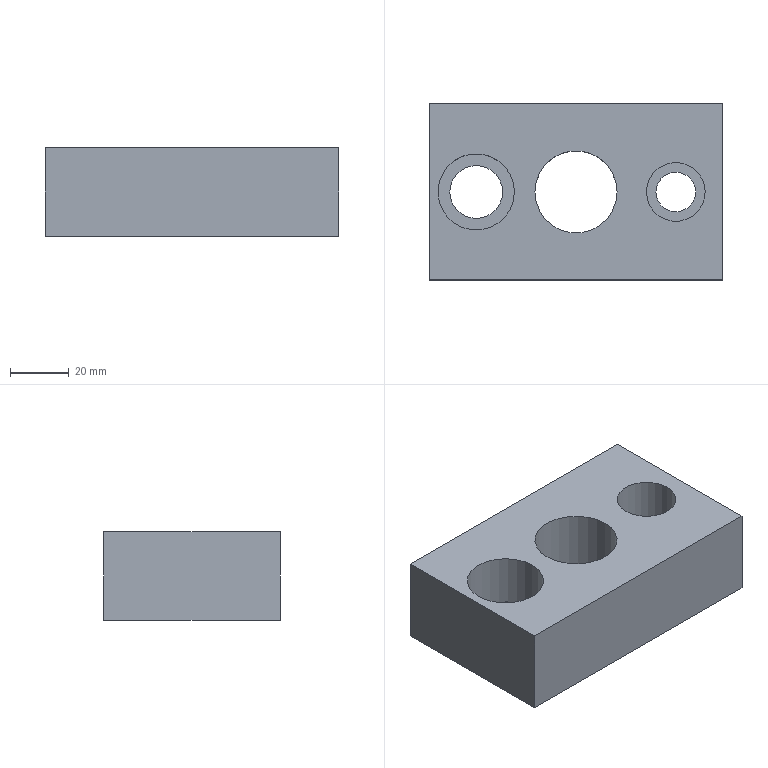Part | STEP file | lll_id4438_x_t | 1 solid | 15 faces | box 100 x 60 x 30 mm | volume 135633 mm3 | plane 9 | cylinder 6 | commonest cylinder face diameters 13.509 x1 18.009 x1 20.008 x1 26.008 x1 28 x1 40 x1
STEP:
#1=CARTESIAN_POINT('',(3051.995,87.,-68.));
#2=VERTEX_POINT('',#1);
#3=CARTESIAN_POINT('',(3061.,87.,-68.));
#4=DIRECTION('',(0.,0.,-1.));
#5=DIRECTION('',(-1.,0.,0.));
#6=AXIS2_PLACEMENT_3D('',#3,#4,#5);
#7=CIRCLE('',#6,9.005);
#8=EDGE_CURVE('',#2,#2,#7,.T.);
#9=ORIENTED_EDGE('',*,*,#8,.F.);
#10=EDGE_LOOP('',(#9));
#11=FACE_BOUND('',#10,.T.);
#12=CARTESIAN_POINT('',(3051.995,87.,-80.));
#13=VERTEX_POINT('',#12);
#14=CARTESIAN_POINT('',(3061.,87.,-80.));
#15=DIRECTION('',(0.,0.,-1.));
#16=DIRECTION('',(-1.,0.,0.));
#17=AXIS2_PLACEMENT_3D('',#14,#15,#16);
#18=CIRCLE('',#17,9.005);
#19=EDGE_CURVE('',#13,#13,#18,.T.);
#20=ORIENTED_EDGE('',*,*,#19,.T.);
#21=EDGE_LOOP('',(#20));
#22=FACE_BOUND('',#21,.T.);
#23=CARTESIAN_POINT('',(3061.,87.,-49.));
#24=DIRECTION('',(0.,0.,-1.));
#25=DIRECTION('',(-1.,0.,0.));
#26=AXIS2_PLACEMENT_3D('',#23,#24,#25);
#27=CYLINDRICAL_SURFACE('',#26,9.005);
#28=ADVANCED_FACE('',(#11,#22),#27,.F.);
#29=CARTESIAN_POINT('',(3074.004,87.,-50.));
#30=VERTEX_POINT('',#29);
#31=CARTESIAN_POINT('',(3061.,87.,-50.));
#32=DIRECTION('',(0.,0.,1.));
#33=DIRECTION('',(1.,0.,0.));
#34=AXIS2_PLACEMENT_3D('',#31,#32,#33);
#35=CIRCLE('',#34,13.004);
#36=EDGE_CURVE('',#30,#30,#35,.T.);
#37=ORIENTED_EDGE('',*,*,#36,.F.);
#38=EDGE_LOOP('',(#37));
#39=FACE_BOUND('',#38,.T.);
#40=CARTESIAN_POINT('',(3081.,87.,-50.));
#41=VERTEX_POINT('',#40);
#42=CARTESIAN_POINT('',(3095.,87.,-50.));
#43=DIRECTION('',(0.,0.,-1.));
#44=DIRECTION('',(-1.,0.,0.));
#45=AXIS2_PLACEMENT_3D('',#42,#43,#44);
#46=CIRCLE('',#45,14.);
#47=EDGE_CURVE('',#41,#41,#46,.T.);
#48=ORIENTED_EDGE('',*,*,#47,.T.);
#49=EDGE_LOOP('',(#48));
#50=FACE_BOUND('',#49,.T.);
#51=CARTESIAN_POINT('',(3118.996,87.,-50.));
#52=VERTEX_POINT('',#51);
#53=CARTESIAN_POINT('',(3129.,87.,-50.));
#54=DIRECTION('',(0.,0.,1.));
#55=DIRECTION('',(-1.,0.,0.));
#56=AXIS2_PLACEMENT_3D('',#53,#54,#55);
#57=CIRCLE('',#56,10.004);
#58=EDGE_CURVE('',#52,#52,#57,.T.);
#59=ORIENTED_EDGE('',*,*,#58,.F.);
#60=EDGE_LOOP('',(#59));
#61=FACE_BOUND('',#60,.T.);
#62=CARTESIAN_POINT('',(3045.,57.,-50.));
#63=VERTEX_POINT('',#62);
#64=CARTESIAN_POINT('',(3145.,57.,-50.));
#65=VERTEX_POINT('',#64);
#66=CARTESIAN_POINT('',(3095.,57.,-50.));
#67=DIRECTION('',(1.,0.,0.));
#68=VECTOR('',#67,1.);
#69=LINE('',#66,#68);
#70=EDGE_CURVE('',#63,#65,#69,.T.);
#71=ORIENTED_EDGE('',*,*,#70,.T.);
#72=CARTESIAN_POINT('',(3145.,117.,-50.));
#73=VERTEX_POINT('',#72);
#74=CARTESIAN_POINT('',(3145.,87.,-50.));
#75=DIRECTION('',(0.,1.,0.));
#76=VECTOR('',#75,1.);
#77=LINE('',#74,#76);
#78=EDGE_CURVE('',#65,#73,#77,.T.);
#79=ORIENTED_EDGE('',*,*,#78,.T.);
#80=CARTESIAN_POINT('',(3045.,117.,-50.));
#81=VERTEX_POINT('',#80);
#82=CARTESIAN_POINT('',(3095.,117.,-50.));
#83=DIRECTION('',(-1.,0.,0.));
#84=VECTOR('',#83,1.);
#85=LINE('',#82,#84);
#86=EDGE_CURVE('',#73,#81,#85,.T.);
#87=ORIENTED_EDGE('',*,*,#86,.T.);
#88=CARTESIAN_POINT('',(3045.,87.,-50.));
#89=DIRECTION('',(0.,-1.,0.));
#90=VECTOR('',#89,1.);
#91=LINE('',#88,#90);
#92=EDGE_CURVE('',#81,#63,#91,.T.);
#93=ORIENTED_EDGE('',*,*,#92,.T.);
#94=EDGE_LOOP('',(#71,#79,#87,#93));
#95=FACE_BOUND('',#94,.T.);
#96=CARTESIAN_POINT('',(3095.,87.,-50.));
#97=DIRECTION('',(0.,0.,1.));
#98=DIRECTION('',(-1.,0.,0.));
#99=AXIS2_PLACEMENT_3D('',#96,#97,#98);
#100=PLANE('',#99);
#101=ADVANCED_FACE('',(#39,#50,#61,#95),#100,.T.);
#102=CARTESIAN_POINT('',(3045.,57.,-80.));
#103=VERTEX_POINT('',#102);
#104=CARTESIAN_POINT('',(3045.,57.,-80.));
#105=DIRECTION('',(0.,0.,1.));
#106=VECTOR('',#105,1.);
#107=LINE('',#104,#106);
#108=EDGE_CURVE('',#103,#63,#107,.T.);
#109=ORIENTED_EDGE('',*,*,#108,.F.);
#110=CARTESIAN_POINT('',(3145.,57.,-80.));
#111=VERTEX_POINT('',#110);
#112=CARTESIAN_POINT('',(3095.,57.,-80.));
#113=DIRECTION('',(-1.,0.,0.));
#114=VECTOR('',#113,1.);
#115=LINE('',#112,#114);
#116=EDGE_CURVE('',#111,#103,#115,.T.);
#117=ORIENTED_EDGE('',*,*,#116,.F.);
#118=CARTESIAN_POINT('',(3145.,57.,-80.));
#119=DIRECTION('',(0.,0.,1.));
#120=VECTOR('',#119,1.);
#121=LINE('',#118,#120);
#122=EDGE_CURVE('',#111,#65,#121,.T.);
#123=ORIENTED_EDGE('',*,*,#122,.T.);
#124=ORIENTED_EDGE('',*,*,#70,.F.);
#125=EDGE_LOOP('',(#109,#117,#123,#124));
#126=FACE_OUTER_BOUND('',#125,.T.);
#127=CARTESIAN_POINT('',(3095.,57.,-80.));
#128=DIRECTION('',(0.,-1.,0.));
#129=DIRECTION('',(0.,0.,-1.));
#130=AXIS2_PLACEMENT_3D('',#127,#128,#129);
#131=PLANE('',#130);
#132=ADVANCED_FACE('',(#126),#131,.T.);
#133=ORIENTED_EDGE('',*,*,#122,.F.);
#134=CARTESIAN_POINT('',(3145.,117.,-80.));
#135=VERTEX_POINT('',#134);
#136=CARTESIAN_POINT('',(3145.,87.,-80.));
#137=DIRECTION('',(0.,-1.,0.));
#138=VECTOR('',#137,1.);
#139=LINE('',#136,#138);
#140=EDGE_CURVE('',#135,#111,#139,.T.);
#141=ORIENTED_EDGE('',*,*,#140,.F.);
#142=CARTESIAN_POINT('',(3145.,117.,-80.));
#143=DIRECTION('',(0.,0.,1.));
#144=VECTOR('',#143,1.);
#145=LINE('',#142,#144);
#146=EDGE_CURVE('',#135,#73,#145,.T.);
#147=ORIENTED_EDGE('',*,*,#146,.T.);
#148=ORIENTED_EDGE('',*,*,#78,.F.);
#149=EDGE_LOOP('',(#133,#141,#147,#148));
#150=FACE_OUTER_BOUND('',#149,.T.);
#151=CARTESIAN_POINT('',(3145.,87.,-80.));
#152=DIRECTION('',(1.,0.,0.));
#153=DIRECTION('',(0.,0.,1.));
#154=AXIS2_PLACEMENT_3D('',#151,#152,#153);
#155=PLANE('',#154);
#156=ADVANCED_FACE('',(#150),#155,.T.);
#157=ORIENTED_EDGE('',*,*,#146,.F.);
#158=CARTESIAN_POINT('',(3045.,117.,-80.));
#159=VERTEX_POINT('',#158);
#160=CARTESIAN_POINT('',(3095.,117.,-80.));
#161=DIRECTION('',(1.,0.,0.));
#162=VECTOR('',#161,1.);
#163=LINE('',#160,#162);
#164=EDGE_CURVE('',#159,#135,#163,.T.);
#165=ORIENTED_EDGE('',*,*,#164,.F.);
#166=CARTESIAN_POINT('',(3045.,117.,-80.));
#167=DIRECTION('',(0.,0.,1.));
#168=VECTOR('',#167,1.);
#169=LINE('',#166,#168);
#170=EDGE_CURVE('',#159,#81,#169,.T.);
#171=ORIENTED_EDGE('',*,*,#170,.T.);
#172=ORIENTED_EDGE('',*,*,#86,.F.);
#173=EDGE_LOOP('',(#157,#165,#171,#172));
#174=FACE_OUTER_BOUND('',#173,.T.);
#175=CARTESIAN_POINT('',(3095.,117.,-80.));
#176=DIRECTION('',(0.,1.,0.));
#177=DIRECTION('',(0.,0.,1.));
#178=AXIS2_PLACEMENT_3D('',#175,#176,#177);
#179=PLANE('',#178);
#180=ADVANCED_FACE('',(#174),#179,.T.);
#181=ORIENTED_EDGE('',*,*,#19,.F.);
#182=EDGE_LOOP('',(#181));
#183=FACE_BOUND('',#182,.T.);
#184=CARTESIAN_POINT('',(3135.755,87.,-80.));
#185=VERTEX_POINT('',#184);
#186=CARTESIAN_POINT('',(3129.,87.,-80.));
#187=DIRECTION('',(0.,0.,1.));
#188=DIRECTION('',(1.,0.,0.));
#189=AXIS2_PLACEMENT_3D('',#186,#187,#188);
#190=CIRCLE('',#189,6.755);
#191=EDGE_CURVE('',#185,#185,#190,.T.);
#192=ORIENTED_EDGE('',*,*,#191,.T.);
#193=EDGE_LOOP('',(#192));
#194=FACE_BOUND('',#193,.T.);
#195=CARTESIAN_POINT('',(3115.,87.,-80.));
#196=VERTEX_POINT('',#195);
#197=CARTESIAN_POINT('',(3095.,87.,-80.));
#198=DIRECTION('',(0.,0.,1.));
#199=DIRECTION('',(1.,0.,0.));
#200=AXIS2_PLACEMENT_3D('',#197,#198,#199);
#201=CIRCLE('',#200,20.);
#202=EDGE_CURVE('',#196,#196,#201,.T.);
#203=ORIENTED_EDGE('',*,*,#202,.T.);
#204=EDGE_LOOP('',(#203));
#205=FACE_BOUND('',#204,.T.);
#206=CARTESIAN_POINT('',(3045.,87.,-80.));
#207=DIRECTION('',(0.,1.,0.));
#208=VECTOR('',#207,1.);
#209=LINE('',#206,#208);
#210=EDGE_CURVE('',#103,#159,#209,.T.);
#211=ORIENTED_EDGE('',*,*,#210,.T.);
#212=ORIENTED_EDGE('',*,*,#164,.T.);
#213=ORIENTED_EDGE('',*,*,#140,.T.);
#214=ORIENTED_EDGE('',*,*,#116,.T.);
#215=EDGE_LOOP('',(#211,#212,#213,#214));
#216=FACE_BOUND('',#215,.T.);
#217=CARTESIAN_POINT('',(3095.,87.,-80.));
#218=DIRECTION('',(0.,0.,-1.));
#219=DIRECTION('',(1.,0.,0.));
#220=AXIS2_PLACEMENT_3D('',#217,#218,#219);
#221=PLANE('',#220);
#222=ADVANCED_FACE('',(#183,#194,#205,#216),#221,.T.);
#223=ORIENTED_EDGE('',*,*,#210,.F.);
#224=ORIENTED_EDGE('',*,*,#108,.T.);
#225=ORIENTED_EDGE('',*,*,#92,.F.);
#226=ORIENTED_EDGE('',*,*,#170,.F.);
#227=EDGE_LOOP('',(#223,#224,#225,#226));
#228=FACE_OUTER_BOUND('',#227,.T.);
#229=CARTESIAN_POINT('',(3045.,87.,-80.));
#230=DIRECTION('',(-1.,0.,0.));
#231=DIRECTION('',(0.,0.,-1.));
#232=AXIS2_PLACEMENT_3D('',#229,#230,#231);
#233=PLANE('',#232);
#234=ADVANCED_FACE('',(#228),#233,.T.);
#235=CARTESIAN_POINT('',(3081.,87.,-70.));
#236=VERTEX_POINT('',#235);
#237=CARTESIAN_POINT('',(3095.,87.,-70.));
#238=DIRECTION('',(0.,0.,-1.));
#239=DIRECTION('',(1.,0.,0.));
#240=AXIS2_PLACEMENT_3D('',#237,#238,#239);
#241=CIRCLE('',#240,14.);
#242=EDGE_CURVE('',#236,#236,#241,.T.);
#243=ORIENTED_EDGE('',*,*,#242,.F.);
#244=EDGE_LOOP('',(#243));
#245=FACE_BOUND('',#244,.T.);
#246=CARTESIAN_POINT('',(3075.,87.,-70.));
#247=VERTEX_POINT('',#246);
#248=CARTESIAN_POINT('',(3095.,87.,-70.));
#249=DIRECTION('',(0.,0.,-1.));
#250=DIRECTION('',(1.,0.,0.));
#251=AXIS2_PLACEMENT_3D('',#248,#249,#250);
#252=CIRCLE('',#251,20.);
#253=EDGE_CURVE('',#247,#247,#252,.T.);
#254=ORIENTED_EDGE('',*,*,#253,.T.);
#255=EDGE_LOOP('',(#254));
#256=FACE_BOUND('',#255,.T.);
#257=CARTESIAN_POINT('',(3095.,87.,-70.));
#258=DIRECTION('',(0.,0.,1.));
#259=DIRECTION('',(-1.,0.,0.));
#260=AXIS2_PLACEMENT_3D('',#257,#258,#259);
#261=PLANE('',#260);
#262=ADVANCED_FACE('',(#245,#256),#261,.F.);
#263=ORIENTED_EDGE('',*,*,#202,.F.);
#264=EDGE_LOOP('',(#263));
#265=FACE_BOUND('',#264,.T.);
#266=ORIENTED_EDGE('',*,*,#253,.F.);
#267=EDGE_LOOP('',(#266));
#268=FACE_BOUND('',#267,.T.);
#269=CARTESIAN_POINT('',(3095.,87.,-75.));
#270=DIRECTION('',(0.,0.,-1.));
#271=DIRECTION('',(-1.,0.,0.));
#272=AXIS2_PLACEMENT_3D('',#269,#270,#271);
#273=CYLINDRICAL_SURFACE('',#272,20.);
#274=ADVANCED_FACE('',(#265,#268),#273,.F.);
#275=ORIENTED_EDGE('',*,*,#191,.F.);
#276=EDGE_LOOP('',(#275));
#277=FACE_BOUND('',#276,.T.);
#278=CARTESIAN_POINT('',(3135.755,87.,-65.));
#279=VERTEX_POINT('',#278);
#280=CARTESIAN_POINT('',(3129.,87.,-65.));
#281=DIRECTION('',(0.,0.,1.));
#282=DIRECTION('',(1.,0.,0.));
#283=AXIS2_PLACEMENT_3D('',#280,#281,#282);
#284=CIRCLE('',#283,6.755);
#285=EDGE_CURVE('',#279,#279,#284,.T.);
#286=ORIENTED_EDGE('',*,*,#285,.T.);
#287=EDGE_LOOP('',(#286));
#288=FACE_BOUND('',#287,.T.);
#289=CARTESIAN_POINT('',(3129.,87.,-48.));
#290=DIRECTION('',(0.,0.,-1.));
#291=DIRECTION('',(-1.,0.,0.));
#292=AXIS2_PLACEMENT_3D('',#289,#290,#291);
#293=CYLINDRICAL_SURFACE('',#292,6.755);
#294=ADVANCED_FACE('',(#277,#288),#293,.F.);
#295=ORIENTED_EDGE('',*,*,#285,.F.);
#296=EDGE_LOOP('',(#295));
#297=FACE_BOUND('',#296,.T.);
#298=CARTESIAN_POINT('',(3118.996,87.,-65.));
#299=VERTEX_POINT('',#298);
#300=CARTESIAN_POINT('',(3129.,87.,-65.));
#301=DIRECTION('',(0.,0.,1.));
#302=DIRECTION('',(-1.,0.,0.));
#303=AXIS2_PLACEMENT_3D('',#300,#301,#302);
#304=CIRCLE('',#303,10.004);
#305=EDGE_CURVE('',#299,#299,#304,.T.);
#306=ORIENTED_EDGE('',*,*,#305,.T.);
#307=EDGE_LOOP('',(#306));
#308=FACE_BOUND('',#307,.T.);
#309=CARTESIAN_POINT('',(3129.,87.,-65.));
#310=DIRECTION('',(0.,0.,-1.));
#311=DIRECTION('',(1.,0.,0.));
#312=AXIS2_PLACEMENT_3D('',#309,#310,#311);
#313=PLANE('',#312);
#314=ADVANCED_FACE('',(#297,#308),#313,.F.);
#315=ORIENTED_EDGE('',*,*,#305,.F.);
#316=EDGE_LOOP('',(#315));
#317=FACE_BOUND('',#316,.T.);
#318=ORIENTED_EDGE('',*,*,#58,.T.);
#319=EDGE_LOOP('',(#318));
#320=FACE_BOUND('',#319,.T.);
#321=CARTESIAN_POINT('',(3129.,87.,-50.));
#322=DIRECTION('',(0.,0.,-1.));
#323=DIRECTION('',(-1.,0.,0.));
#324=AXIS2_PLACEMENT_3D('',#321,#322,#323);
#325=CYLINDRICAL_SURFACE('',#324,10.004);
#326=ADVANCED_FACE('',(#317,#320),#325,.F.);
#327=ORIENTED_EDGE('',*,*,#47,.F.);
#328=EDGE_LOOP('',(#327));
#329=FACE_BOUND('',#328,.T.);
#330=ORIENTED_EDGE('',*,*,#242,.T.);
#331=EDGE_LOOP('',(#330));
#332=FACE_BOUND('',#331,.T.);
#333=CARTESIAN_POINT('',(3095.,87.,-8.));
#334=DIRECTION('',(0.,0.,-1.));
#335=DIRECTION('',(-1.,0.,0.));
#336=AXIS2_PLACEMENT_3D('',#333,#334,#335);
#337=CYLINDRICAL_SURFACE('',#336,14.);
#338=ADVANCED_FACE('',(#329,#332),#337,.F.);
#339=ORIENTED_EDGE('',*,*,#8,.T.);
#340=EDGE_LOOP('',(#339));
#341=FACE_BOUND('',#340,.T.);
#342=CARTESIAN_POINT('',(3074.004,87.,-68.));
#343=VERTEX_POINT('',#342);
#344=CARTESIAN_POINT('',(3061.,87.,-68.));
#345=DIRECTION('',(0.,0.,-1.));
#346=DIRECTION('',(1.,0.,0.));
#347=AXIS2_PLACEMENT_3D('',#344,#345,#346);
#348=CIRCLE('',#347,13.004);
#349=EDGE_CURVE('',#343,#343,#348,.T.);
#350=ORIENTED_EDGE('',*,*,#349,.F.);
#351=EDGE_LOOP('',(#350));
#352=FACE_BOUND('',#351,.T.);
#353=CARTESIAN_POINT('',(3061.,87.,-68.));
#354=DIRECTION('',(0.,0.,-1.));
#355=DIRECTION('',(1.,0.,0.));
#356=AXIS2_PLACEMENT_3D('',#353,#354,#355);
#357=PLANE('',#356);
#358=ADVANCED_FACE('',(#341,#352),#357,.F.);
#359=ORIENTED_EDGE('',*,*,#36,.T.);
#360=EDGE_LOOP('',(#359));
#361=FACE_BOUND('',#360,.T.);
#362=ORIENTED_EDGE('',*,*,#349,.T.);
#363=EDGE_LOOP('',(#362));
#364=FACE_BOUND('',#363,.T.);
#365=CARTESIAN_POINT('',(3061.,87.,-49.));
#366=DIRECTION('',(0.,0.,-1.));
#367=DIRECTION('',(-1.,0.,0.));
#368=AXIS2_PLACEMENT_3D('',#365,#366,#367);
#369=CYLINDRICAL_SURFACE('',#368,13.004);
#370=ADVANCED_FACE('',(#361,#364),#369,.F.);
#371=CLOSED_SHELL('',(#28,#101,#132,#156,#180,#222,#234,#262,#274,#294,#314,#326,#338,#358,#370));
#372=MANIFOLD_SOLID_BREP('',#371);
#373=(LENGTH_UNIT()NAMED_UNIT(*)SI_UNIT(.MILLI.,.METRE.));
#374=UNCERTAINTY_MEASURE_WITH_UNIT(LENGTH_MEASURE(0.00002),#373,'','');
#375=(NAMED_UNIT(*)PLANE_ANGLE_UNIT()SI_UNIT($,.RADIAN.));
#376=PLANE_ANGLE_MEASURE_WITH_UNIT(PLANE_ANGLE_MEASURE(0.01745),#375);
#377=DIMENSIONAL_EXPONENTS(0.,0.,0.,0.,0.,0.,0.);
#378=(CONVERSION_BASED_UNIT('DEGREE',#376)NAMED_UNIT(#377)PLANE_ANGLE_UNIT());
#379=(NAMED_UNIT(*)SI_UNIT($,.STERADIAN.)SOLID_ANGLE_UNIT());
#380=(GEOMETRIC_REPRESENTATION_CONTEXT(3)GLOBAL_UNCERTAINTY_ASSIGNED_CONTEXT((#374))GLOBAL_UNIT_ASSIGNED_CONTEXT((#373,#378,#379))REPRESENTATION_CONTEXT('',''));
#381=ADVANCED_BREP_SHAPE_REPRESENTATION('',(#372),#380);